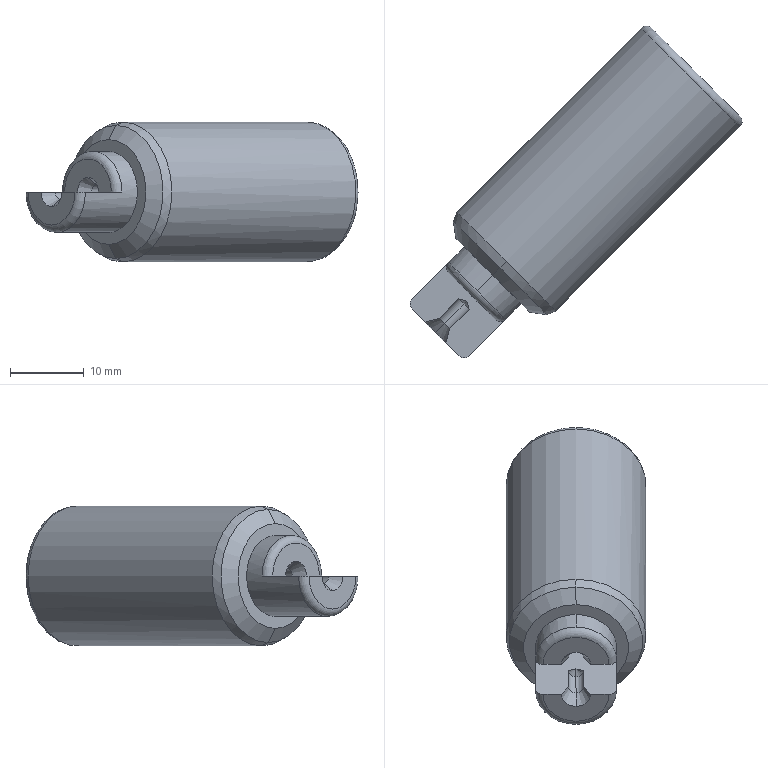Part | STEP file | 1_id1754_x_t | 1 solid | 174 faces | box 45.134 x 45.134 x 19 mm | volume 11498 mm3 | plane 115 | other 35 | cone 12 | cylinder 9 | torus 3 | commonest cylinder face diameters 2 x4 4.9 x2 11 x2 19 x1